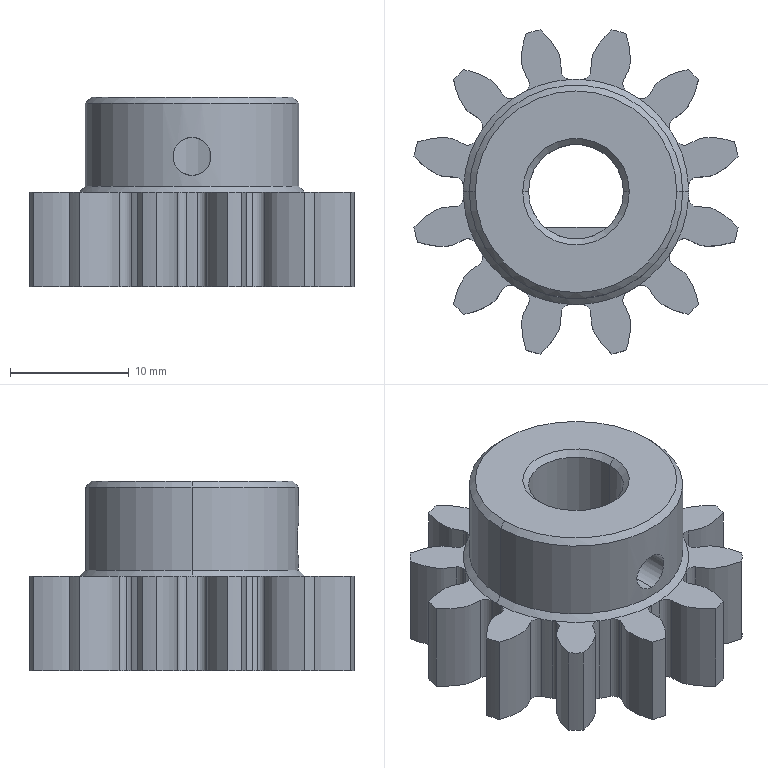Part | SolidWorks | features ICE 5, Chamfer 2, CirPattern 1, Extrusion 1, RefAxis 1 | 1 solid | 107 faces | box 27.338 x 27.338 x 16 mm | volume 4690 mm3 | cylinder 61 | spline 24 | plane 16 | cone 6 | commonest cylinder face diameters 1.52 x30 19 x13 28 x12 3.2 x2 8 x2 18 x2